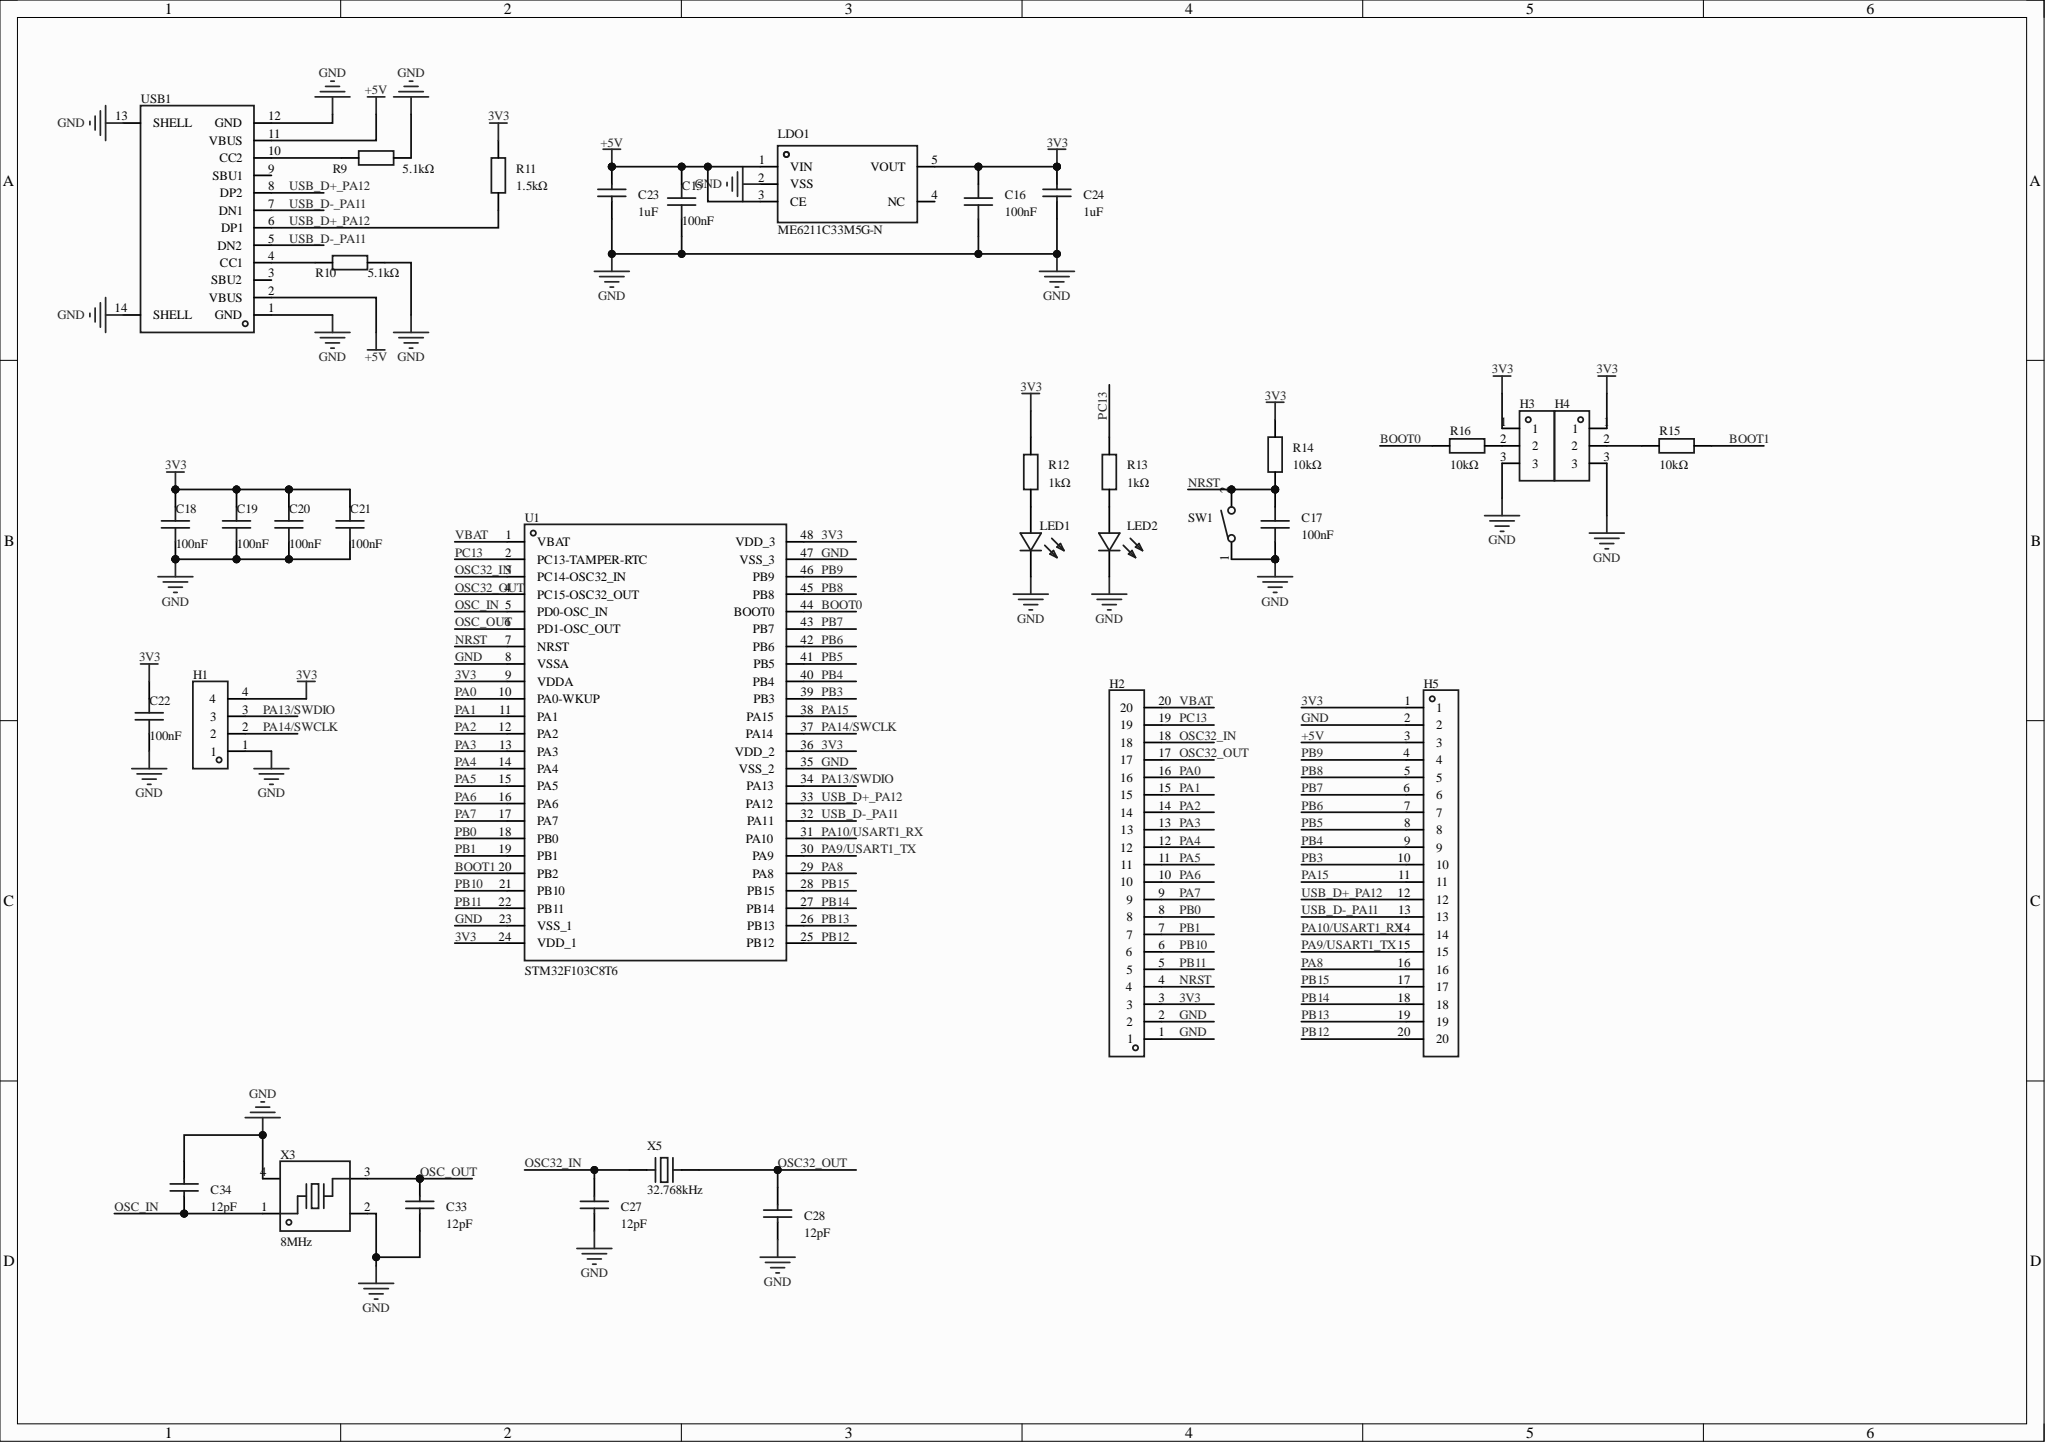Circuit board | Altium Designer | 35 parts | 49 nets
Bill of materials:
Comment,Description,Designator,Footprint,LibRef,Quantity
"100nF","容值:100nF;精度:±10%;额定电压:50V;温度系数:X7R;","C15, C16, C17, C18, C19, C20, C21, C22","C0402","GRM155R71H104KE14D","8"
"1uF","容值:1uF;精度:±10%;额定电压:10V;温度系数:X5R;","C23, C24","C0402","CL05A105KP5NNNC","2"
"12pF","容值:12pF;精度:±5%;额定电压:50V;温度系数:C0G;","C27, C28, C33, C34","C0402","0402CG120J500NT","4"
"DZ254W-11-04-65","插针结构:1x4P;间距:2.54mm;行距:-;圆针/方针:方针;安装方式:弯插;排数:单排;总PIN位数:4P;额定电流:3A;额定电压:-;配合针长度:6mm;塑高:2.54mm;端接针长度:-;触头材质:黄铜;触头镀层:金;工作温度:-;颜色:黑色;","H1","HDR-TH_4P-P2.54-H-M-W10.3","DZ254W-11-04-65","1"
"2.54-1*20P直针","插针结构:1x20P;间距:2.54mm;行距:-;圆针/方针:方针;安装方式:直插;排数:单排;总PIN位数:20P;额定电流:3A;额定电压:-;配合针长度:-;塑高:-;端接针长度:-;触头材质:黄铜;触头镀层:-;工作温度:-40℃~+105℃;颜色:黑色;","H2, H5","HDR-TH_20P-P2.54-V-M-1","2.54-1*20P直针","2"
"PZ254V-11-03P","插针结构:1x3P;间距:2.54mm;行距:-;圆针/方针:方针;安装方式:直插;排数:单排;总PIN位数:3P;额定电流:3A;额定电压:250V;配合针长度:6mm;塑高:2.5mm;端接针长度:3mm;工作温度:-40℃~+105℃;颜色:黑色;","H3, H4","HDR-TH_3P-P2.54-V-M_PZ254V-11-03P","PZ254V-11-03P","2"
"ME6211C33M5G-N","输出类型:固定;工作电压:6V;输出电压:3.3V;输出电流:500mA;电源纹波抑制比(PSRR):70dB@(1kHz);输出极性:正极;","LDO1","SOT-23-5_L3.0-W1.7-P0.95-LS2.8-BL","ME6211C33M5G-N","1"
"NCD0603R1","灯头类型:-;发光颜色:红色;正向压降(Vf):1.6V~2.6V;功率:65mW;正向电流:25mA;波长:615nm~630nm;二极管配置:独立二极管;透镜颜色:-;色温:-;发光强度:220mcd;发光角度:130°;载带方式:-;工作温度:-30℃~+85℃;","LED1","LED0603-RD_RED","NCD0603R1_C84263","1"
"NCD0603B1","灯头类型:-;发光颜色:蓝色;正向压降(Vf):2.6V~3.6V;功率:72mW;正向电流:10mA;波长:463nm~475nm;二极管配置:独立二极管;透镜颜色:-;色温:-;发光强度:220mcd;发光角度:130°;载带方式:-;工作温度:-30℃~+85℃;","LED2","LED0603-RD","NCD0603B1","1"
"5.1kΩ","","R9, R10","R0805","Res_0805","2"
"1.5kΩ","","R11","R0805","Res_0805","1"
"1kΩ","","R12, R13","R0805","Res_0805","2"
"10kΩ","","R14, R15, R16","R0805","Res_0805","3"
"TS-1101-B-W","电路结构:单刀单掷;按钮形状:矩形按钮;作用力:1.6N;安装方式:立贴;开关长度:6mm;开关宽度:3.6mm;开关高度:2.5mm;带支架:不带支架;触点电流:50mA;额定电压:12V;带灯:无;工作寿命:5万次;","SW1","KEY-SMD_2P-L6.0-W3.6-P7.4-LS8.0-L","TS-1101-B-W_C500065","1"
"STM32F103C8T6","CPU内核:ARM-M3;CPU最大主频:72MHz;应用领域:-;","U1","LQFP-48_L7.0-W7.0-P0.50-LS9.0-BL","STM32F103C8T6","1"
"TYPE-C 16PIN 2MD(073)","连接器类型:Type-C;协议标准:-;公母:母;安装方式:卧贴;触点数量:16P;端口数量:1;额定电流 - 电源:3A;工作温度:-25℃~+85℃;","USB1","USB-C-SMD_TYPE-C-6PIN-2MD-073","TYPE-C 16PIN 2MD(073)","1"
"8MHz","晶振类型:贴片晶振;频率:8MHz;常温频差:±10ppm;负载电容:12pF;频率稳定度:±20ppm;","X3","CRYSTAL-SMD_4P-L3.2-W2.5-BL-1","XL2EL89COI-111YLC-8M","1"
"32.768kHz","晶振类型:贴片晶振;频率:32.768kHz;常温频差:±20ppm;负载电容:12.5pF;频率稳定度:±30ppm;","X5","OSC-SMD_L3.2-W1.5","X321532768KGD2SI","1"
Netlist (Protel format):
[
C15
C0402
100nF



]
[
C16
C0402
100nF



]
[
C17
C0402
100nF



]
[
C18
C0402
100nF



]
[
C19
C0402
100nF



]
[
C20
C0402
100nF



]
[
C21
C0402
100nF



]
[
C22
C0402
100nF



]
[
C23
C0402
1uF



]
[
C24
C0402
1uF



]
[
C27
C0402
12pF



]
[
C28
C0402
12pF



]
[
C33
C0402
12pF



]
[
C34
C0402
12pF



]
[
H1
HDR-TH_4P-P2.54-H-M-W10.3
DZ254W-11-04-65



]
[
H2
HDR-TH_20P-P2.54-V-M-1
2.54-1*20P直针



]
[
H3
HDR-TH_3P-P2.54-V-M_PZ254V-11-03P
PZ254V-11-03P



]
[
H4
HDR-TH_3P-P2.54-V-M_PZ254V-11-03P
PZ254V-11-03P



]
[
H5
HDR-TH_20P-P2.54-V-M-1
2.54-1*20P直针



]
[
LDO1
SOT-23-5_L3.0-W1.7-P0.95-LS2.8-BL
ME6211C33M5G-N



]
[
LED1
LED0603-RD_RED
NCD0603R1



]
[
LED2
LED0603-RD
NCD0603B1



]
[
R9
R0805
5.1kΩ



]
[
R10
R0805
5.1kΩ



]
[
R11
R0805
1.5kΩ



]
[
R12
R0805
1kΩ



]
[
R13
R0805
1kΩ



]
[
R14
R0805
10kΩ



]
[
R15
R0805
10kΩ



]
[
R16
R0805
10kΩ



]
[
SW1
KEY-SMD_2P-L6.0-W3.6-P7.4-LS8.0-L
TS-1101-B-W



]
[
U1
LQFP-48_L7.0-W7.0-P0.50-LS9.0-BL
STM32F103C8T6



]
[
USB1
USB-C-SMD_TYPE-C-6PIN-2MD-073
TYPE-C 16PIN 2MD(073)



]
[
X3
CRYSTAL-SMD_4P-L3.2-W2.5-BL-1
8MHz



]
[
X5
OSC-SMD_L3.2-W1.5
32.768kHz



]
(
VBAT
H2-20
U1-1
)
(
USB_D-_PA11
H5-13
U1-32
USB1-5
USB1-7
)
(
USB_D+_PA12
H5-12
R11-1
U1-33
USB1-6
USB1-8
)
(
PC13
H2-19
R13-2
U1-2
)
(
PB15
H5-17
U1-28
)
(
PB14
H5-18
U1-27
)
(
PB13
H5-19
U1-26
)
(
PB12
H5-20
U1-25
)
(
PB11
H2-5
U1-22
)
(
PB10
H2-6
U1-21
)
(
PB9
H5-4
U1-46
)
(
PB8
H5-5
U1-45
)
(
PB7
H5-6
U1-43
)
(
PB6
H5-7
U1-42
)
(
PB5
H5-8
U1-41
)
(
PB4
H5-9
U1-40
)
(
PB3
H5-10
U1-39
)
(
PB1
H2-7
U1-19
)
(
PB0
H2-8
U1-18
)
(
PA15
H5-11
U1-38
)
(
PA14/SWCLK
H1-2
U1-37
)
(
PA13/SWDIO
H1-3
U1-34
)
(
PA10/USART1_RX
H5-14
U1-31
)
(
PA9/USART1_TX
H5-15
U1-30
)
(
PA8
H5-16
U1-29
)
(
PA7
H2-9
U1-17
)
(
PA6
H2-10
U1-16
)
(
PA5
H2-11
U1-15
)
(
PA4
H2-12
U1-14
)
(
PA3
H2-13
U1-13
)
(
PA2
H2-14
U1-12
)
(
PA1
H2-15
U1-11
)
(
PA0
H2-16
U1-10
)
(
OSC_OUT
C33-2
U1-6
X3-3
)
(
OSC_IN
C34-1
U1-5
X3-1
)
(
OSC32_OUT
C28-2
H2-17
U1-4
X5-2
)
(
OSC32_IN
C27-2
H2-18
U1-3
X5-1
)
(
NRST
C17-2
H2-4
R14-1
SW1-2
U1-7
)
(
NetR10_1
R10-1
USB1-4
)
(
NetR9_1
R9-1
USB1-10
)
(
NetLED2_2
LED2-2
R13-1
)
(
NetLED1_2
LED1-2
R12-1
)
(
NetH4_2
H4-2
R15-1
)
(
NetH3_2
H3-2
R16-2
)
(
GND
C15-1
C16-1
C17-1
C18-1
C19-1
C20-1
C21-1
C22-1
C23-1
C24-1
C27-1
C28-1
C33-1
C34-2
H1-1
H2-1
H2-2
H3-3
H4-3
H5-2
LDO1-2
LED1-1
LED2-1
R9-2
R10-2
SW1-1
U1-8
U1-23
U1-35
U1-47
USB1-1
USB1-12
USB1-13
USB1-14
X3-2
X3-4
)
(
BOOT1
R15-2
U1-20
)
(
BOOT0
R16-1
U1-44
)
(
+5V
C15-2
C23-2
H5-3
LDO1-1
LDO1-3
USB1-2
USB1-11
)
(
3V3
C16-2
C18-2
C19-2
C20-2
C21-2
C22-2
C24-2
H1-4
H2-3
H3-1
H4-1
H5-1
LDO1-5
R11-2
R12-2
R14-2
U1-9
U1-24
U1-36
U1-48
)